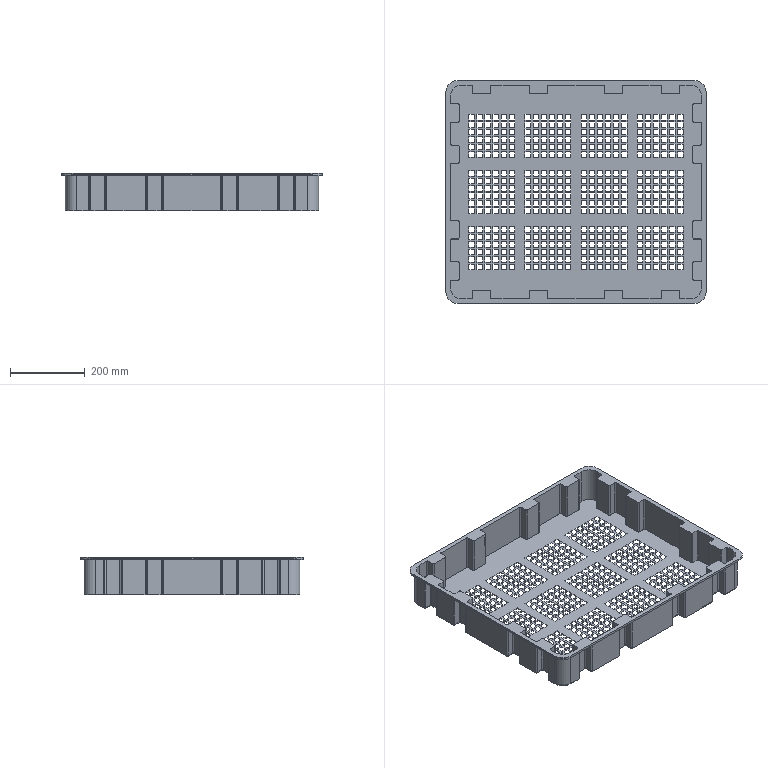Part | SolidWorks | features ICE 5, Fillet 3, Extrusion 1, Shell 1 | 1 solid | 2158 faces | box 695 x 595 x 100 mm | volume 1469602 mm3 | plane 1946 | cylinder 212 | commonest cylinder face diameters 6 x128 2 x32 10 x32 60 x16 56 x4